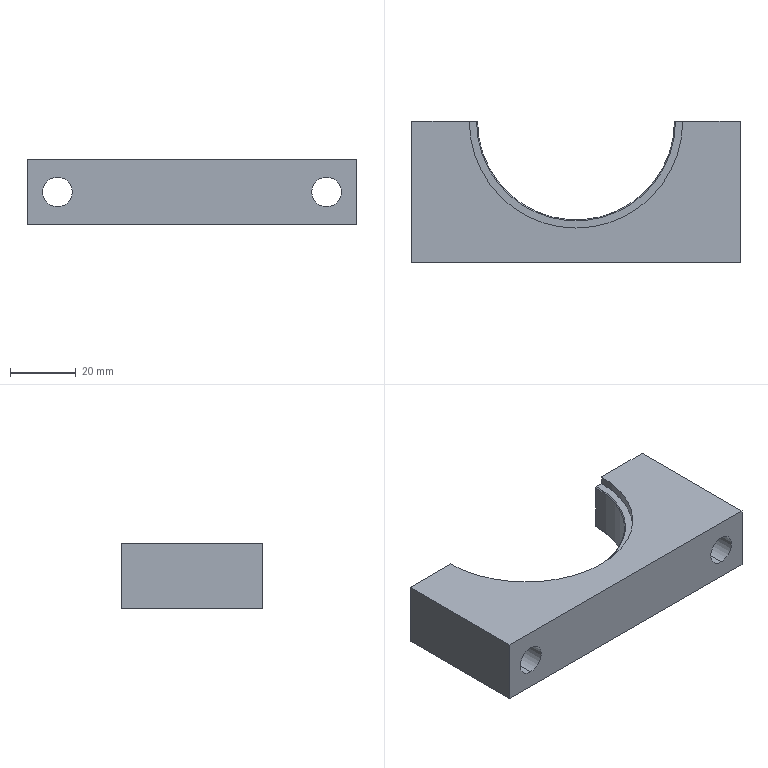Part | SolidWorks | features HoleWzd 2, ICE 2, Chamfer 1, Extrusion 1 | 1 solid | 21 faces | box 100 x 43 x 20 mm | volume 50968 mm3 | plane 10 | cylinder 9 | cone 2 | commonest cylinder face diameters 9 x4 4 x2 65 x2 60 x1
STEP:
#1=CARTESIAN_POINT('',(0.,-34.,8.));
#2=VERTEX_POINT('',#1);
#3=CARTESIAN_POINT('',(0.,-34.,12.));
#4=VERTEX_POINT('',#3);
#5=CARTESIAN_POINT('',(0.,-34.,10.));
#6=DIRECTION('',(0.,1.,0.));
#7=DIRECTION('',(0.,0.,1.));
#8=AXIS2_PLACEMENT_3D('',#5,#6,#7);
#9=CIRCLE('',#8,2.);
#10=EDGE_CURVE('',#2,#4,#9,.T.);
#11=ORIENTED_EDGE('',*,*,#10,.F.);
#12=CARTESIAN_POINT('',(0.,-30.,8.));
#13=VERTEX_POINT('',#12);
#14=CARTESIAN_POINT('',(0.,0.,8.));
#15=DIRECTION('',(0.,1.,0.));
#16=VECTOR('',#15,1000.);
#17=LINE('',#14,#16);
#18=EDGE_CURVE('',#2,#13,#17,.T.);
#19=ORIENTED_EDGE('',*,*,#18,.T.);
#20=CARTESIAN_POINT('',(0.,-30.,12.));
#21=VERTEX_POINT('',#20);
#22=CARTESIAN_POINT('',(0.,-30.,12.));
#23=CARTESIAN_POINT('',(-0.1322,-30.,12.));
#24=CARTESIAN_POINT('',(-0.2622,-29.999,11.987));
#25=CARTESIAN_POINT('',(-0.5178,-29.996,11.936));
#26=CARTESIAN_POINT('',(-0.6449,-29.993,11.898));
#27=CARTESIAN_POINT('',(-0.8871,-29.987,11.797));
#28=CARTESIAN_POINT('',(-1.002,-29.983,11.736));
#29=CARTESIAN_POINT('',(-1.219,-29.975,11.591));
#30=CARTESIAN_POINT('',(-1.322,-29.971,11.506));
#31=CARTESIAN_POINT('',(-1.599,-29.958,11.229));
#32=CARTESIAN_POINT('',(-1.748,-29.949,11.006));
#33=CARTESIAN_POINT('',(-1.947,-29.937,10.525));
#34=CARTESIAN_POINT('',(-2.,-29.933,10.262));
#35=CARTESIAN_POINT('',(-2.,-29.933,9.87));
#36=CARTESIAN_POINT('',(-1.987,-29.934,9.738));
#37=CARTESIAN_POINT('',(-1.936,-29.937,9.481));
#38=CARTESIAN_POINT('',(-1.898,-29.94,9.356));
#39=CARTESIAN_POINT('',(-1.798,-29.946,9.114));
#40=CARTESIAN_POINT('',(-1.735,-29.95,8.997));
#41=CARTESIAN_POINT('',(-1.591,-29.958,8.78));
#42=CARTESIAN_POINT('',(-1.508,-29.962,8.679));
#43=CARTESIAN_POINT('',(-1.321,-29.971,8.493));
#44=CARTESIAN_POINT('',(-1.22,-29.975,8.41));
#45=CARTESIAN_POINT('',(-1.003,-29.983,8.265));
#46=CARTESIAN_POINT('',(-0.8865,-29.987,8.202));
#47=CARTESIAN_POINT('',(-0.6442,-29.993,8.102));
#48=CARTESIAN_POINT('',(-0.5195,-29.996,8.064));
#49=CARTESIAN_POINT('',(-0.2631,-29.999,8.013));
#50=CARTESIAN_POINT('',(-0.1305,-30.,8.));
#51=CARTESIAN_POINT('',(0.,-30.,8.));
#52=B_SPLINE_CURVE_WITH_KNOTS('',3,(#22,#23,#24,#25,#26,#27,#28,#29,#30,#31,#32,#33,#34,#35,#36,#37,#38,#39,#40,#41,#42,#43,#44,#45,#46,#47,#48,#49,#50,#51),.UNSPECIFIED.,.F.,.F.,(4,2,2,2,2,2,2,2,2,2,2,2,2,2,4),(0.,0.0003909,0.0007818,0.001173,0.001564,0.002345,0.003127,0.003518,0.003909,0.0043,0.004691,0.005082,0.005473,0.005864,0.006255),.UNSPECIFIED.);
#53=EDGE_CURVE('',#21,#13,#52,.T.);
#54=ORIENTED_EDGE('',*,*,#53,.F.);
#55=CARTESIAN_POINT('',(0.,0.,12.));
#56=DIRECTION('',(0.,1.,0.));
#57=VECTOR('',#56,1000.);
#58=LINE('',#55,#57);
#59=EDGE_CURVE('',#4,#21,#58,.T.);
#60=ORIENTED_EDGE('',*,*,#59,.F.);
#61=EDGE_LOOP('',(#11,#19,#54,#60));
#62=FACE_OUTER_BOUND('',#61,.T.);
#63=CARTESIAN_POINT('',(0.,0.,10.));
#64=DIRECTION('',(0.,1.,0.));
#65=DIRECTION('',(0.,0.,1.));
#66=AXIS2_PLACEMENT_3D('',#63,#64,#65);
#67=CYLINDRICAL_SURFACE('',#66,2.);
#68=ADVANCED_FACE('',(#62),#67,.F.);
#69=CARTESIAN_POINT('',(-41.,-43.,5.5));
#70=VERTEX_POINT('',#69);
#71=CARTESIAN_POINT('',(-41.,-43.,14.5));
#72=VERTEX_POINT('',#71);
#73=CARTESIAN_POINT('',(-41.,-43.,10.));
#74=DIRECTION('',(0.,1.,0.));
#75=DIRECTION('',(0.,0.,1.));
#76=AXIS2_PLACEMENT_3D('',#73,#74,#75);
#77=CIRCLE('',#76,4.5);
#78=EDGE_CURVE('',#70,#72,#77,.T.);
#79=ORIENTED_EDGE('',*,*,#78,.F.);
#80=CARTESIAN_POINT('',(-41.,0.,5.5));
#81=VERTEX_POINT('',#80);
#82=CARTESIAN_POINT('',(-41.,0.,5.5));
#83=DIRECTION('',(0.,1.,0.));
#84=VECTOR('',#83,1000.);
#85=LINE('',#82,#84);
#86=EDGE_CURVE('',#70,#81,#85,.T.);
#87=ORIENTED_EDGE('',*,*,#86,.T.);
#88=CARTESIAN_POINT('',(-41.,0.,14.5));
#89=VERTEX_POINT('',#88);
#90=CARTESIAN_POINT('',(-41.,0.,10.));
#91=DIRECTION('',(0.,1.,0.));
#92=DIRECTION('',(0.,0.,1.));
#93=AXIS2_PLACEMENT_3D('',#90,#91,#92);
#94=CIRCLE('',#93,4.5);
#95=EDGE_CURVE('',#81,#89,#94,.T.);
#96=ORIENTED_EDGE('',*,*,#95,.T.);
#97=CARTESIAN_POINT('',(-41.,0.,14.5));
#98=DIRECTION('',(0.,1.,0.));
#99=VECTOR('',#98,1000.);
#100=LINE('',#97,#99);
#101=EDGE_CURVE('',#72,#89,#100,.T.);
#102=ORIENTED_EDGE('',*,*,#101,.F.);
#103=EDGE_LOOP('',(#79,#87,#96,#102));
#104=FACE_OUTER_BOUND('',#103,.T.);
#105=CARTESIAN_POINT('',(-41.,0.,10.));
#106=DIRECTION('',(0.,1.,0.));
#107=DIRECTION('',(0.,0.,1.));
#108=AXIS2_PLACEMENT_3D('',#105,#106,#107);
#109=CYLINDRICAL_SURFACE('',#108,4.5);
#110=ADVANCED_FACE('',(#104),#109,.F.);
#111=CARTESIAN_POINT('',(41.,-43.,5.5));
#112=VERTEX_POINT('',#111);
#113=CARTESIAN_POINT('',(41.,-43.,14.5));
#114=VERTEX_POINT('',#113);
#115=CARTESIAN_POINT('',(41.,-43.,10.));
#116=DIRECTION('',(0.,1.,0.));
#117=DIRECTION('',(0.,0.,1.));
#118=AXIS2_PLACEMENT_3D('',#115,#116,#117);
#119=CIRCLE('',#118,4.5);
#120=EDGE_CURVE('',#112,#114,#119,.T.);
#121=ORIENTED_EDGE('',*,*,#120,.F.);
#122=CARTESIAN_POINT('',(41.,0.,5.5));
#123=VERTEX_POINT('',#122);
#124=CARTESIAN_POINT('',(41.,0.,5.5));
#125=DIRECTION('',(0.,1.,0.));
#126=VECTOR('',#125,1000.);
#127=LINE('',#124,#126);
#128=EDGE_CURVE('',#112,#123,#127,.T.);
#129=ORIENTED_EDGE('',*,*,#128,.T.);
#130=CARTESIAN_POINT('',(41.,0.,14.5));
#131=VERTEX_POINT('',#130);
#132=CARTESIAN_POINT('',(41.,0.,10.));
#133=DIRECTION('',(0.,1.,0.));
#134=DIRECTION('',(0.,0.,1.));
#135=AXIS2_PLACEMENT_3D('',#132,#133,#134);
#136=CIRCLE('',#135,4.5);
#137=EDGE_CURVE('',#123,#131,#136,.T.);
#138=ORIENTED_EDGE('',*,*,#137,.T.);
#139=CARTESIAN_POINT('',(41.,0.,14.5));
#140=DIRECTION('',(0.,1.,0.));
#141=VECTOR('',#140,1000.);
#142=LINE('',#139,#141);
#143=EDGE_CURVE('',#114,#131,#142,.T.);
#144=ORIENTED_EDGE('',*,*,#143,.F.);
#145=EDGE_LOOP('',(#121,#129,#138,#144));
#146=FACE_OUTER_BOUND('',#145,.T.);
#147=CARTESIAN_POINT('',(41.,0.,10.));
#148=DIRECTION('',(0.,1.,0.));
#149=DIRECTION('',(0.,0.,1.));
#150=AXIS2_PLACEMENT_3D('',#147,#148,#149);
#151=CYLINDRICAL_SURFACE('',#150,4.5);
#152=ADVANCED_FACE('',(#146),#151,.F.);
#153=CARTESIAN_POINT('',(30.3,0.,2.5));
#154=VERTEX_POINT('',#153);
#155=CARTESIAN_POINT('',(32.5,0.,2.5));
#156=VERTEX_POINT('',#155);
#157=CARTESIAN_POINT('',(30.,0.,2.5));
#158=DIRECTION('',(1.,0.,0.));
#159=VECTOR('',#158,1000.);
#160=LINE('',#157,#159);
#161=EDGE_CURVE('',#154,#156,#160,.T.);
#162=ORIENTED_EDGE('',*,*,#161,.F.);
#163=CARTESIAN_POINT('',(30.,0.,2.8));
#164=VERTEX_POINT('',#163);
#165=CARTESIAN_POINT('',(0.,0.,32.8));
#166=DIRECTION('',(-0.7071,0.,0.7071));
#167=VECTOR('',#166,1000.);
#168=LINE('',#165,#167);
#169=EDGE_CURVE('',#154,#164,#168,.T.);
#170=ORIENTED_EDGE('',*,*,#169,.T.);
#171=CARTESIAN_POINT('',(30.,0.,17.2));
#172=VERTEX_POINT('',#171);
#173=CARTESIAN_POINT('',(30.,0.,20.));
#174=DIRECTION('',(0.,0.,-1.));
#175=VECTOR('',#174,1000.);
#176=LINE('',#173,#175);
#177=EDGE_CURVE('',#172,#164,#176,.T.);
#178=ORIENTED_EDGE('',*,*,#177,.F.);
#179=CARTESIAN_POINT('',(30.3,0.,17.5));
#180=VERTEX_POINT('',#179);
#181=CARTESIAN_POINT('',(0.,0.,-12.8));
#182=DIRECTION('',(0.7071,0.,0.7071));
#183=VECTOR('',#182,1000.);
#184=LINE('',#181,#183);
#185=EDGE_CURVE('',#172,#180,#184,.T.);
#186=ORIENTED_EDGE('',*,*,#185,.T.);
#187=CARTESIAN_POINT('',(32.5,0.,17.5));
#188=VERTEX_POINT('',#187);
#189=CARTESIAN_POINT('',(30.,0.,17.5));
#190=DIRECTION('',(-1.,0.,0.));
#191=VECTOR('',#190,1000.);
#192=LINE('',#189,#191);
#193=EDGE_CURVE('',#188,#180,#192,.T.);
#194=ORIENTED_EDGE('',*,*,#193,.F.);
#195=CARTESIAN_POINT('',(32.5,0.,20.));
#196=VERTEX_POINT('',#195);
#197=CARTESIAN_POINT('',(32.5,0.,17.5));
#198=DIRECTION('',(0.,0.,1.));
#199=VECTOR('',#198,1000.);
#200=LINE('',#197,#199);
#201=EDGE_CURVE('',#188,#196,#200,.T.);
#202=ORIENTED_EDGE('',*,*,#201,.T.);
#203=CARTESIAN_POINT('',(50.,0.,20.));
#204=VERTEX_POINT('',#203);
#205=CARTESIAN_POINT('',(30.,0.,20.));
#206=DIRECTION('',(-1.,0.,0.));
#207=VECTOR('',#206,1000.);
#208=LINE('',#205,#207);
#209=EDGE_CURVE('',#204,#196,#208,.T.);
#210=ORIENTED_EDGE('',*,*,#209,.F.);
#211=CARTESIAN_POINT('',(50.,0.,0.));
#212=VERTEX_POINT('',#211);
#213=CARTESIAN_POINT('',(50.,0.,20.));
#214=DIRECTION('',(0.,0.,-1.));
#215=VECTOR('',#214,1000.);
#216=LINE('',#213,#215);
#217=EDGE_CURVE('',#204,#212,#216,.T.);
#218=ORIENTED_EDGE('',*,*,#217,.T.);
#219=CARTESIAN_POINT('',(32.5,0.,0.));
#220=VERTEX_POINT('',#219);
#221=CARTESIAN_POINT('',(30.,0.,0.));
#222=DIRECTION('',(-1.,0.,0.));
#223=VECTOR('',#222,1000.);
#224=LINE('',#221,#223);
#225=EDGE_CURVE('',#212,#220,#224,.T.);
#226=ORIENTED_EDGE('',*,*,#225,.T.);
#227=CARTESIAN_POINT('',(32.5,0.,2.5));
#228=DIRECTION('',(0.,0.,1.));
#229=VECTOR('',#228,1000.);
#230=LINE('',#227,#229);
#231=EDGE_CURVE('',#220,#156,#230,.T.);
#232=ORIENTED_EDGE('',*,*,#231,.T.);
#233=EDGE_LOOP('',(#162,#170,#178,#186,#194,#202,#210,#218,#226,#232));
#234=FACE_OUTER_BOUND('',#233,.T.);
#235=CARTESIAN_POINT('',(41.,0.,10.));
#236=DIRECTION('',(0.,1.,0.));
#237=DIRECTION('',(0.,0.,1.));
#238=AXIS2_PLACEMENT_3D('',#235,#236,#237);
#239=CIRCLE('',#238,4.5);
#240=EDGE_CURVE('',#131,#123,#239,.T.);
#241=ORIENTED_EDGE('',*,*,#240,.F.);
#242=ORIENTED_EDGE('',*,*,#137,.F.);
#243=EDGE_LOOP('',(#241,#242));
#244=FACE_BOUND('',#243,.T.);
#245=CARTESIAN_POINT('',(30.,0.,20.));
#246=DIRECTION('',(0.,-1.,0.));
#247=DIRECTION('',(1.,0.,0.));
#248=AXIS2_PLACEMENT_3D('',#245,#246,#247);
#249=PLANE('',#248);
#250=ADVANCED_FACE('',(#234,#244),#249,.F.);
#251=ORIENTED_EDGE('',*,*,#53,.T.);
#252=CARTESIAN_POINT('',(0.,-30.,8.));
#253=CARTESIAN_POINT('',(0.261,-30.,8.));
#254=CARTESIAN_POINT('',(0.5242,-29.996,8.052));
#255=CARTESIAN_POINT('',(1.006,-29.984,8.252));
#256=CARTESIAN_POINT('',(1.229,-29.975,8.401));
#257=CARTESIAN_POINT('',(1.505,-29.962,8.677));
#258=CARTESIAN_POINT('',(1.59,-29.958,8.78));
#259=CARTESIAN_POINT('',(1.735,-29.95,8.997));
#260=CARTESIAN_POINT('',(1.797,-29.946,9.112));
#261=CARTESIAN_POINT('',(1.897,-29.94,9.354));
#262=CARTESIAN_POINT('',(1.936,-29.937,9.481));
#263=CARTESIAN_POINT('',(1.987,-29.934,9.737));
#264=CARTESIAN_POINT('',(2.,-29.933,9.866));
#265=CARTESIAN_POINT('',(2.,-29.933,10.13));
#266=CARTESIAN_POINT('',(1.987,-29.934,10.261));
#267=CARTESIAN_POINT('',(1.937,-29.937,10.516));
#268=CARTESIAN_POINT('',(1.898,-29.94,10.643));
#269=CARTESIAN_POINT('',(1.798,-29.946,10.886));
#270=CARTESIAN_POINT('',(1.737,-29.95,11.001));
#271=CARTESIAN_POINT('',(1.592,-29.958,11.218));
#272=CARTESIAN_POINT('',(1.507,-29.962,11.321));
#273=CARTESIAN_POINT('',(1.323,-29.971,11.506));
#274=CARTESIAN_POINT('',(1.222,-29.975,11.588));
#275=CARTESIAN_POINT('',(1.004,-29.983,11.735));
#276=CARTESIAN_POINT('',(0.8877,-29.987,11.797));
#277=CARTESIAN_POINT('',(0.5269,-29.996,11.947));
#278=CARTESIAN_POINT('',(0.2643,-30.,12.));
#279=CARTESIAN_POINT('',(0.,-30.,12.));
#280=B_SPLINE_CURVE_WITH_KNOTS('',3,(#252,#253,#254,#255,#256,#257,#258,#259,#260,#261,#262,#263,#264,#265,#266,#267,#268,#269,#270,#271,#272,#273,#274,#275,#276,#277,#278,#279),.UNSPECIFIED.,.F.,.F.,(4,2,2,2,2,2,2,2,2,2,2,2,2,4),(0.006255,0.007036,0.007818,0.008209,0.0086,0.00899,0.009381,0.009772,0.01016,0.01055,0.01094,0.01134,0.01173,0.01251),.UNSPECIFIED.);
#281=EDGE_CURVE('',#13,#21,#280,.T.);
#282=ORIENTED_EDGE('',*,*,#281,.T.);
#283=EDGE_LOOP('',(#251,#282));
#284=FACE_BOUND('',#283,.T.);
#285=ORIENTED_EDGE('',*,*,#177,.T.);
#286=CARTESIAN_POINT('',(-30.,0.,2.8));
#287=VERTEX_POINT('',#286);
#288=CARTESIAN_POINT('',(0.,0.,2.8));
#289=DIRECTION('',(0.,0.,-1.));
#290=DIRECTION('',(-1.,0.,0.));
#291=AXIS2_PLACEMENT_3D('',#288,#289,#290);
#292=CIRCLE('',#291,30.);
#293=EDGE_CURVE('',#164,#287,#292,.T.);
#294=ORIENTED_EDGE('',*,*,#293,.T.);
#295=CARTESIAN_POINT('',(-30.,0.,17.2));
#296=VERTEX_POINT('',#295);
#297=CARTESIAN_POINT('',(-30.,0.,20.));
#298=DIRECTION('',(0.,0.,-1.));
#299=VECTOR('',#298,1000.);
#300=LINE('',#297,#299);
#301=EDGE_CURVE('',#296,#287,#300,.T.);
#302=ORIENTED_EDGE('',*,*,#301,.F.);
#303=CARTESIAN_POINT('',(0.,0.,17.2));
#304=DIRECTION('',(0.,0.,1.));
#305=DIRECTION('',(1.,0.,0.));
#306=AXIS2_PLACEMENT_3D('',#303,#304,#305);
#307=CIRCLE('',#306,30.);
#308=EDGE_CURVE('',#296,#172,#307,.T.);
#309=ORIENTED_EDGE('',*,*,#308,.T.);
#310=EDGE_LOOP('',(#285,#294,#302,#309));
#311=FACE_OUTER_BOUND('',#310,.T.);
#312=CARTESIAN_POINT('',(0.,0.,20.));
#313=DIRECTION('',(0.,0.,-1.));
#314=DIRECTION('',(-1.,0.,0.));
#315=AXIS2_PLACEMENT_3D('',#312,#313,#314);
#316=CYLINDRICAL_SURFACE('',#315,30.);
#317=ADVANCED_FACE('',(#284,#311),#316,.F.);
#318=CARTESIAN_POINT('',(-41.,0.,10.));
#319=DIRECTION('',(0.,1.,0.));
#320=DIRECTION('',(0.,0.,1.));
#321=AXIS2_PLACEMENT_3D('',#318,#319,#320);
#322=CIRCLE('',#321,4.5);
#323=EDGE_CURVE('',#89,#81,#322,.T.);
#324=ORIENTED_EDGE('',*,*,#323,.F.);
#325=ORIENTED_EDGE('',*,*,#95,.F.);
#326=EDGE_LOOP('',(#324,#325));
#327=FACE_BOUND('',#326,.T.);
#328=ORIENTED_EDGE('',*,*,#301,.T.);
#329=CARTESIAN_POINT('',(-30.3,0.,2.5));
#330=VERTEX_POINT('',#329);
#331=CARTESIAN_POINT('',(0.,0.,32.8));
#332=DIRECTION('',(-0.7071,0.,-0.7071));
#333=VECTOR('',#332,1000.);
#334=LINE('',#331,#333);
#335=EDGE_CURVE('',#287,#330,#334,.T.);
#336=ORIENTED_EDGE('',*,*,#335,.T.);
#337=CARTESIAN_POINT('',(-32.5,0.,2.5));
#338=VERTEX_POINT('',#337);
#339=CARTESIAN_POINT('',(-50.,0.,2.5));
#340=DIRECTION('',(1.,0.,0.));
#341=VECTOR('',#340,1000.);
#342=LINE('',#339,#341);
#343=EDGE_CURVE('',#338,#330,#342,.T.);
#344=ORIENTED_EDGE('',*,*,#343,.F.);
#345=CARTESIAN_POINT('',(-32.5,0.,0.));
#346=VERTEX_POINT('',#345);
#347=CARTESIAN_POINT('',(-32.5,0.,2.5));
#348=DIRECTION('',(0.,0.,-1.));
#349=VECTOR('',#348,1000.);
#350=LINE('',#347,#349);
#351=EDGE_CURVE('',#338,#346,#350,.T.);
#352=ORIENTED_EDGE('',*,*,#351,.T.);
#353=CARTESIAN_POINT('',(-50.,0.,0.));
#354=VERTEX_POINT('',#353);
#355=CARTESIAN_POINT('',(-50.,0.,0.));
#356=DIRECTION('',(-1.,0.,0.));
#357=VECTOR('',#356,1000.);
#358=LINE('',#355,#357);
#359=EDGE_CURVE('',#346,#354,#358,.T.);
#360=ORIENTED_EDGE('',*,*,#359,.T.);
#361=CARTESIAN_POINT('',(-50.,0.,20.));
#362=VERTEX_POINT('',#361);
#363=CARTESIAN_POINT('',(-50.,0.,20.));
#364=DIRECTION('',(0.,0.,-1.));
#365=VECTOR('',#364,1000.);
#366=LINE('',#363,#365);
#367=EDGE_CURVE('',#362,#354,#366,.T.);
#368=ORIENTED_EDGE('',*,*,#367,.F.);
#369=CARTESIAN_POINT('',(-32.5,0.,20.));
#370=VERTEX_POINT('',#369);
#371=CARTESIAN_POINT('',(-50.,0.,20.));
#372=DIRECTION('',(-1.,0.,0.));
#373=VECTOR('',#372,1000.);
#374=LINE('',#371,#373);
#375=EDGE_CURVE('',#370,#362,#374,.T.);
#376=ORIENTED_EDGE('',*,*,#375,.F.);
#377=CARTESIAN_POINT('',(-32.5,0.,17.5));
#378=VERTEX_POINT('',#377);
#379=CARTESIAN_POINT('',(-32.5,0.,17.5));
#380=DIRECTION('',(0.,0.,-1.));
#381=VECTOR('',#380,1000.);
#382=LINE('',#379,#381);
#383=EDGE_CURVE('',#370,#378,#382,.T.);
#384=ORIENTED_EDGE('',*,*,#383,.T.);
#385=CARTESIAN_POINT('',(-30.3,0.,17.5));
#386=VERTEX_POINT('',#385);
#387=CARTESIAN_POINT('',(-50.,0.,17.5));
#388=DIRECTION('',(-1.,0.,0.));
#389=VECTOR('',#388,1000.);
#390=LINE('',#387,#389);
#391=EDGE_CURVE('',#386,#378,#390,.T.);
#392=ORIENTED_EDGE('',*,*,#391,.F.);
#393=CARTESIAN_POINT('',(0.,0.,-12.8));
#394=DIRECTION('',(0.7071,0.,-0.7071));
#395=VECTOR('',#394,1000.);
#396=LINE('',#393,#395);
#397=EDGE_CURVE('',#386,#296,#396,.T.);
#398=ORIENTED_EDGE('',*,*,#397,.T.);
#399=EDGE_LOOP('',(#328,#336,#344,#352,#360,#368,#376,#384,#392,#398));
#400=FACE_OUTER_BOUND('',#399,.T.);
#401=CARTESIAN_POINT('',(-50.,0.,20.));
#402=DIRECTION('',(0.,-1.,0.));
#403=DIRECTION('',(1.,0.,0.));
#404=AXIS2_PLACEMENT_3D('',#401,#402,#403);
#405=PLANE('',#404);
#406=ADVANCED_FACE('',(#327,#400),#405,.F.);
#407=CARTESIAN_POINT('',(-50.,-43.,0.));
#408=VERTEX_POINT('',#407);
#409=CARTESIAN_POINT('',(-50.,-43.,0.));
#410=DIRECTION('',(0.,-1.,0.));
#411=VECTOR('',#410,1000.);
#412=LINE('',#409,#411);
#413=EDGE_CURVE('',#354,#408,#412,.T.);
#414=ORIENTED_EDGE('',*,*,#413,.T.);
#415=CARTESIAN_POINT('',(-50.,-43.,20.));
#416=VERTEX_POINT('',#415);
#417=CARTESIAN_POINT('',(-50.,-43.,20.));
#418=DIRECTION('',(0.,0.,-1.));
#419=VECTOR('',#418,1000.);
#420=LINE('',#417,#419);
#421=EDGE_CURVE('',#416,#408,#420,.T.);
#422=ORIENTED_EDGE('',*,*,#421,.F.);
#423=CARTESIAN_POINT('',(-50.,-43.,20.));
#424=DIRECTION('',(0.,-1.,0.));
#425=VECTOR('',#424,1000.);
#426=LINE('',#423,#425);
#427=EDGE_CURVE('',#362,#416,#426,.T.);
#428=ORIENTED_EDGE('',*,*,#427,.F.);
#429=ORIENTED_EDGE('',*,*,#367,.T.);
#430=EDGE_LOOP('',(#414,#422,#428,#429));
#431=FACE_OUTER_BOUND('',#430,.T.);
#432=CARTESIAN_POINT('',(-50.,-43.,20.));
#433=DIRECTION('',(1.,0.,0.));
#434=DIRECTION('',(0.,0.,-1.));
#435=AXIS2_PLACEMENT_3D('',#432,#433,#434);
#436=PLANE('',#435);
#437=ADVANCED_FACE('',(#431),#436,.F.);
#438=CARTESIAN_POINT('',(-41.,-43.,10.));
#439=DIRECTION('',(0.,1.,0.));
#440=DIRECTION('',(0.,0.,1.));
#441=AXIS2_PLACEMENT_3D('',#438,#439,#440);
#442=CIRCLE('',#441,4.5);
#443=EDGE_CURVE('',#72,#70,#442,.T.);
#444=ORIENTED_EDGE('',*,*,#443,.T.);
#445=ORIENTED_EDGE('',*,*,#78,.T.);
#446=EDGE_LOOP('',(#444,#445));
#447=FACE_BOUND('',#446,.T.);
#448=CARTESIAN_POINT('',(41.,-43.,10.));
#449=DIRECTION('',(0.,1.,0.));
#450=DIRECTION('',(0.,0.,1.));
#451=AXIS2_PLACEMENT_3D('',#448,#449,#450);
#452=CIRCLE('',#451,4.5);
#453=EDGE_CURVE('',#114,#112,#452,.T.);
#454=ORIENTED_EDGE('',*,*,#453,.T.);
#455=ORIENTED_EDGE('',*,*,#120,.T.);
#456=EDGE_LOOP('',(#454,#455));
#457=FACE_BOUND('',#456,.T.);
#458=CARTESIAN_POINT('',(50.,-43.,0.));
#459=VERTEX_POINT('',#458);
#460=CARTESIAN_POINT('',(-50.,-43.,0.));
#461=DIRECTION('',(1.,0.,0.));
#462=VECTOR('',#461,1000.);
#463=LINE('',#460,#462);
#464=EDGE_CURVE('',#408,#459,#463,.T.);
#465=ORIENTED_EDGE('',*,*,#464,.T.);
#466=CARTESIAN_POINT('',(50.,-43.,20.));
#467=VERTEX_POINT('',#466);
#468=CARTESIAN_POINT('',(50.,-43.,20.));
#469=DIRECTION('',(0.,0.,-1.));
#470=VECTOR('',#469,1000.);
#471=LINE('',#468,#470);
#472=EDGE_CURVE('',#467,#459,#471,.T.);
#473=ORIENTED_EDGE('',*,*,#472,.F.);
#474=CARTESIAN_POINT('',(-50.,-43.,20.));
#475=DIRECTION('',(1.,0.,0.));
#476=VECTOR('',#475,1000.);
#477=LINE('',#474,#476);
#478=EDGE_CURVE('',#416,#467,#477,.T.);
#479=ORIENTED_EDGE('',*,*,#478,.F.);
#480=ORIENTED_EDGE('',*,*,#421,.T.);
#481=EDGE_LOOP('',(#465,#473,#479,#480));
#482=FACE_OUTER_BOUND('',#481,.T.);
#483=CARTESIAN_POINT('',(-50.,-43.,20.));
#484=DIRECTION('',(0.,1.,0.));
#485=DIRECTION('',(-1.,0.,0.));
#486=AXIS2_PLACEMENT_3D('',#483,#484,#485);
#487=PLANE('',#486);
#488=ADVANCED_FACE('',(#447,#457,#482),#487,.F.);
#489=CARTESIAN_POINT('',(50.,-43.,0.));
#490=DIRECTION('',(0.,1.,0.));
#491=VECTOR('',#490,1000.);
#492=LINE('',#489,#491);
#493=EDGE_CURVE('',#459,#212,#492,.T.);
#494=ORIENTED_EDGE('',*,*,#493,.T.);
#495=ORIENTED_EDGE('',*,*,#217,.F.);
#496=CARTESIAN_POINT('',(50.,-43.,20.));
#497=DIRECTION('',(0.,1.,0.));
#498=VECTOR('',#497,1000.);
#499=LINE('',#496,#498);
#500=EDGE_CURVE('',#467,#204,#499,.T.);
#501=ORIENTED_EDGE('',*,*,#500,.F.);
#502=ORIENTED_EDGE('',*,*,#472,.T.);
#503=EDGE_LOOP('',(#494,#495,#501,#502));
#504=FACE_OUTER_BOUND('',#503,.T.);
#505=CARTESIAN_POINT('',(50.,-43.,20.));
#506=DIRECTION('',(-1.,0.,0.));
#507=DIRECTION('',(0.,-1.,0.));
#508=AXIS2_PLACEMENT_3D('',#505,#506,#507);
#509=PLANE('',#508);
#510=ADVANCED_FACE('',(#504),#509,.F.);
#511=CARTESIAN_POINT('',(0.,0.,20.));
#512=DIRECTION('',(0.,0.,1.));
#513=DIRECTION('',(1.,0.,0.));
#514=AXIS2_PLACEMENT_3D('',#511,#512,#513);
#515=CIRCLE('',#514,32.5);
#516=EDGE_CURVE('',#370,#196,#515,.T.);
#517=ORIENTED_EDGE('',*,*,#516,.F.);
#518=ORIENTED_EDGE('',*,*,#375,.T.);
#519=ORIENTED_EDGE('',*,*,#427,.T.);
#520=ORIENTED_EDGE('',*,*,#478,.T.);
#521=ORIENTED_EDGE('',*,*,#500,.T.);
#522=ORIENTED_EDGE('',*,*,#209,.T.);
#523=EDGE_LOOP('',(#517,#518,#519,#520,#521,#522));
#524=FACE_OUTER_BOUND('',#523,.T.);
#525=CARTESIAN_POINT('',(0.,0.,20.));
#526=DIRECTION('',(0.,0.,1.));
#527=DIRECTION('',(1.,0.,0.));
#528=AXIS2_PLACEMENT_3D('',#525,#526,#527);
#529=PLANE('',#528);
#530=ADVANCED_FACE('',(#524),#529,.T.);
#531=ORIENTED_EDGE('',*,*,#359,.F.);
#532=CARTESIAN_POINT('',(0.,0.,0.));
#533=DIRECTION('',(0.,0.,1.));
#534=DIRECTION('',(1.,0.,0.));
#535=AXIS2_PLACEMENT_3D('',#532,#533,#534);
#536=CIRCLE('',#535,32.5);
#537=EDGE_CURVE('',#346,#220,#536,.T.);
#538=ORIENTED_EDGE('',*,*,#537,.T.);
#539=ORIENTED_EDGE('',*,*,#225,.F.);
#540=ORIENTED_EDGE('',*,*,#493,.F.);
#541=ORIENTED_EDGE('',*,*,#464,.F.);
#542=ORIENTED_EDGE('',*,*,#413,.F.);
#543=EDGE_LOOP('',(#531,#538,#539,#540,#541,#542));
#544=FACE_OUTER_BOUND('',#543,.T.);
#545=CARTESIAN_POINT('',(0.,0.,0.));
#546=DIRECTION('',(0.,0.,1.));
#547=DIRECTION('',(1.,0.,0.));
#548=AXIS2_PLACEMENT_3D('',#545,#546,#547);
#549=PLANE('',#548);
#550=ADVANCED_FACE('',(#544),#549,.F.);
#551=ORIENTED_EDGE('',*,*,#193,.T.);
#552=CARTESIAN_POINT('',(0.,0.,17.5));
#553=DIRECTION('',(0.,0.,-1.));
#554=DIRECTION('',(1.,0.,0.));
#555=AXIS2_PLACEMENT_3D('',#552,#553,#554);
#556=CIRCLE('',#555,30.3);
#557=EDGE_CURVE('',#180,#386,#556,.T.);
#558=ORIENTED_EDGE('',*,*,#557,.T.);
#559=ORIENTED_EDGE('',*,*,#391,.T.);
#560=CARTESIAN_POINT('',(0.,0.,17.5));
#561=DIRECTION('',(0.,0.,1.));
#562=DIRECTION('',(1.,0.,0.));
#563=AXIS2_PLACEMENT_3D('',#560,#561,#562);
#564=CIRCLE('',#563,32.5);
#565=EDGE_CURVE('',#378,#188,#564,.T.);
#566=ORIENTED_EDGE('',*,*,#565,.T.);
#567=EDGE_LOOP('',(#551,#558,#559,#566));
#568=FACE_OUTER_BOUND('',#567,.T.);
#569=CARTESIAN_POINT('',(0.,0.,17.5));
#570=DIRECTION('',(0.,0.,1.));
#571=DIRECTION('',(1.,0.,0.));
#572=AXIS2_PLACEMENT_3D('',#569,#570,#571);
#573=PLANE('',#572);
#574=ADVANCED_FACE('',(#568),#573,.T.);
#575=ORIENTED_EDGE('',*,*,#516,.T.);
#576=ORIENTED_EDGE('',*,*,#201,.F.);
#577=ORIENTED_EDGE('',*,*,#565,.F.);
#578=ORIENTED_EDGE('',*,*,#383,.F.);
#579=EDGE_LOOP('',(#575,#576,#577,#578));
#580=FACE_OUTER_BOUND('',#579,.T.);
#581=CARTESIAN_POINT('',(0.,0.,17.5));
#582=DIRECTION('',(0.,0.,1.));
#583=DIRECTION('',(1.,0.,0.));
#584=AXIS2_PLACEMENT_3D('',#581,#582,#583);
#585=CYLINDRICAL_SURFACE('',#584,32.5);
#586=ADVANCED_FACE('',(#580),#585,.F.);
#587=ORIENTED_EDGE('',*,*,#343,.T.);
#588=CARTESIAN_POINT('',(0.,0.,2.5));
#589=DIRECTION('',(0.,0.,1.));
#590=DIRECTION('',(-1.,0.,0.));
#591=AXIS2_PLACEMENT_3D('',#588,#589,#590);
#592=CIRCLE('',#591,30.3);
#593=EDGE_CURVE('',#330,#154,#592,.T.);
#594=ORIENTED_EDGE('',*,*,#593,.T.);
#595=ORIENTED_EDGE('',*,*,#161,.T.);
#596=CARTESIAN_POINT('',(0.,0.,2.5));
#597=DIRECTION('',(0.,0.,-1.));
#598=DIRECTION('',(-1.,0.,0.));
#599=AXIS2_PLACEMENT_3D('',#596,#597,#598);
#600=CIRCLE('',#599,32.5);
#601=EDGE_CURVE('',#156,#338,#600,.T.);
#602=ORIENTED_EDGE('',*,*,#601,.T.);
#603=EDGE_LOOP('',(#587,#594,#595,#602));
#604=FACE_OUTER_BOUND('',#603,.T.);
#605=CARTESIAN_POINT('',(0.,0.,2.5));
#606=DIRECTION('',(0.,0.,-1.));
#607=DIRECTION('',(-1.,0.,0.));
#608=AXIS2_PLACEMENT_3D('',#605,#606,#607);
#609=PLANE('',#608);
#610=ADVANCED_FACE('',(#604),#609,.T.);
#611=ORIENTED_EDGE('',*,*,#601,.F.);
#612=ORIENTED_EDGE('',*,*,#231,.F.);
#613=ORIENTED_EDGE('',*,*,#537,.F.);
#614=ORIENTED_EDGE('',*,*,#351,.F.);
#615=EDGE_LOOP('',(#611,#612,#613,#614));
#616=FACE_OUTER_BOUND('',#615,.T.);
#617=CARTESIAN_POINT('',(0.,0.,2.5));
#618=DIRECTION('',(0.,0.,-1.));
#619=DIRECTION('',(-1.,0.,0.));
#620=AXIS2_PLACEMENT_3D('',#617,#618,#619);
#621=CYLINDRICAL_SURFACE('',#620,32.5);
#622=ADVANCED_FACE('',(#616),#621,.F.);
#623=ORIENTED_EDGE('',*,*,#335,.F.);
#624=ORIENTED_EDGE('',*,*,#293,.F.);
#625=ORIENTED_EDGE('',*,*,#169,.F.);
#626=ORIENTED_EDGE('',*,*,#593,.F.);
#627=EDGE_LOOP('',(#623,#624,#625,#626));
#628=FACE_OUTER_BOUND('',#627,.T.);
#629=CARTESIAN_POINT('',(0.,0.,2.5));
#630=DIRECTION('',(0.,0.,-1.));
#631=DIRECTION('',(-1.,0.,0.));
#632=AXIS2_PLACEMENT_3D('',#629,#630,#631);
#633=CONICAL_SURFACE('',#632,30.3,0.7854);
#634=ADVANCED_FACE('',(#628),#633,.F.);
#635=ORIENTED_EDGE('',*,*,#185,.F.);
#636=ORIENTED_EDGE('',*,*,#308,.F.);
#637=ORIENTED_EDGE('',*,*,#397,.F.);
#638=ORIENTED_EDGE('',*,*,#557,.F.);
#639=EDGE_LOOP('',(#635,#636,#637,#638));
#640=FACE_OUTER_BOUND('',#639,.T.);
#641=CARTESIAN_POINT('',(0.,0.,17.5));
#642=DIRECTION('',(0.,0.,1.));
#643=DIRECTION('',(1.,0.,0.));
#644=AXIS2_PLACEMENT_3D('',#641,#642,#643);
#645=CONICAL_SURFACE('',#644,30.3,0.7854);
#646=ADVANCED_FACE('',(#640),#645,.F.);
#647=ORIENTED_EDGE('',*,*,#128,.F.);
#648=ORIENTED_EDGE('',*,*,#453,.F.);
#649=ORIENTED_EDGE('',*,*,#143,.T.);
#650=ORIENTED_EDGE('',*,*,#240,.T.);
#651=EDGE_LOOP('',(#647,#648,#649,#650));
#652=FACE_OUTER_BOUND('',#651,.T.);
#653=CARTESIAN_POINT('',(41.,0.,10.));
#654=DIRECTION('',(0.,1.,0.));
#655=DIRECTION('',(0.,0.,1.));
#656=AXIS2_PLACEMENT_3D('',#653,#654,#655);
#657=CYLINDRICAL_SURFACE('',#656,4.5);
#658=ADVANCED_FACE('',(#652),#657,.F.);
#659=ORIENTED_EDGE('',*,*,#86,.F.);
#660=ORIENTED_EDGE('',*,*,#443,.F.);
#661=ORIENTED_EDGE('',*,*,#101,.T.);
#662=ORIENTED_EDGE('',*,*,#323,.T.);
#663=EDGE_LOOP('',(#659,#660,#661,#662));
#664=FACE_OUTER_BOUND('',#663,.T.);
#665=CARTESIAN_POINT('',(-41.,0.,10.));
#666=DIRECTION('',(0.,1.,0.));
#667=DIRECTION('',(0.,0.,1.));
#668=AXIS2_PLACEMENT_3D('',#665,#666,#667);
#669=CYLINDRICAL_SURFACE('',#668,4.5);
#670=ADVANCED_FACE('',(#664),#669,.F.);
#671=ORIENTED_EDGE('',*,*,#18,.F.);
#672=CARTESIAN_POINT('',(0.,-34.,10.));
#673=DIRECTION('',(0.,1.,0.));
#674=DIRECTION('',(0.,0.,1.));
#675=AXIS2_PLACEMENT_3D('',#672,#673,#674);
#676=CIRCLE('',#675,2.);
#677=EDGE_CURVE('',#4,#2,#676,.T.);
#678=ORIENTED_EDGE('',*,*,#677,.F.);
#679=ORIENTED_EDGE('',*,*,#59,.T.);
#680=ORIENTED_EDGE('',*,*,#281,.F.);
#681=EDGE_LOOP('',(#671,#678,#679,#680));
#682=FACE_OUTER_BOUND('',#681,.T.);
#683=CARTESIAN_POINT('',(0.,0.,10.));
#684=DIRECTION('',(0.,1.,0.));
#685=DIRECTION('',(0.,0.,1.));
#686=AXIS2_PLACEMENT_3D('',#683,#684,#685);
#687=CYLINDRICAL_SURFACE('',#686,2.);
#688=ADVANCED_FACE('',(#682),#687,.F.);
#689=ORIENTED_EDGE('',*,*,#677,.T.);
#690=ORIENTED_EDGE('',*,*,#10,.T.);
#691=EDGE_LOOP('',(#689,#690));
#692=FACE_OUTER_BOUND('',#691,.T.);
#693=CARTESIAN_POINT('',(0.,-34.,10.));
#694=DIRECTION('',(0.,-1.,0.));
#695=DIRECTION('',(0.,0.,-1.));
#696=AXIS2_PLACEMENT_3D('',#693,#694,#695);
#697=PLANE('',#696);
#698=ADVANCED_FACE('',(#692),#697,.F.);
#699=CLOSED_SHELL('',(#68,#110,#152,#250,#317,#406,#437,#488,#510,#530,#550,#574,#586,#610,#622,#634,#646,#658,#670,#688,#698));
#700=MANIFOLD_SOLID_BREP('',#699);
#701=CARTESIAN_POINT('',(0.,0.,0.));
#702=DIRECTION('',(0.,0.,1.));
#703=DIRECTION('',(1.,0.,0.));
#704=AXIS2_PLACEMENT_3D('',#701,#702,#703);
#705=(LENGTH_UNIT()NAMED_UNIT(*)SI_UNIT(.MILLI.,.METRE.));
#706=UNCERTAINTY_MEASURE_WITH_UNIT(LENGTH_MEASURE(0.00001),#705,'','');
#707=(NAMED_UNIT(*)PLANE_ANGLE_UNIT()SI_UNIT($,.RADIAN.));
#708=(NAMED_UNIT(*)SI_UNIT($,.STERADIAN.)SOLID_ANGLE_UNIT());
#709=(GEOMETRIC_REPRESENTATION_CONTEXT(3)GLOBAL_UNCERTAINTY_ASSIGNED_CONTEXT((#706))GLOBAL_UNIT_ASSIGNED_CONTEXT((#705,#707,#708))REPRESENTATION_CONTEXT('',''));
#710=ADVANCED_BREP_SHAPE_REPRESENTATION('',(#700,#704),#709);